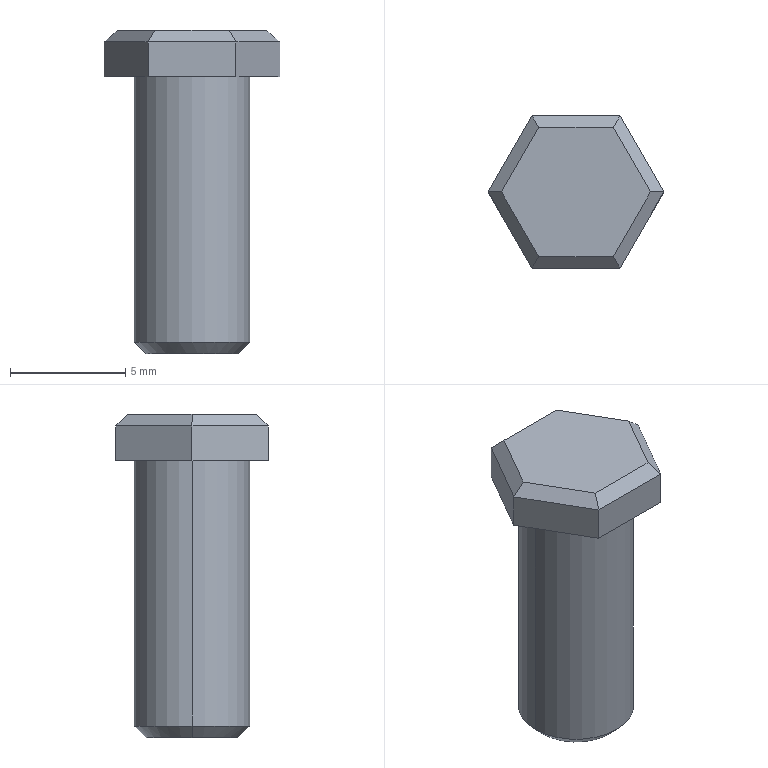Part | SolidWorks | features Chamfer 1, Extrusion 1, ICE 1 | 1 solid | 19 faces | box 7.616 x 6.595 x 14 mm | volume 306.418 mm3 | plane 15 | cone 2 | cylinder 2 | commonest cylinder face diameters 5 x2
STEP:
#1=CARTESIAN_POINT('',(718.,45.,-12.));
#2=VERTEX_POINT('',#1);
#3=CARTESIAN_POINT('',(722.,45.,-12.));
#4=VERTEX_POINT('',#3);
#5=CARTESIAN_POINT('',(720.,45.,-12.));
#6=DIRECTION('',(0.,0.,-1.));
#7=DIRECTION('',(1.,0.,0.));
#8=AXIS2_PLACEMENT_3D('',#5,#6,#7);
#9=CIRCLE('',#8,2.);
#10=EDGE_CURVE('',#2,#4,#9,.T.);
#11=ORIENTED_EDGE('',*,*,#10,.F.);
#12=CARTESIAN_POINT('',(717.5,45.,-11.5));
#13=VERTEX_POINT('',#12);
#14=CARTESIAN_POINT('',(717.5,45.,-11.5));
#15=DIRECTION('',(-0.7071,0.,0.7071));
#16=VECTOR('',#15,1000.);
#17=LINE('',#14,#16);
#18=EDGE_CURVE('',#2,#13,#17,.T.);
#19=ORIENTED_EDGE('',*,*,#18,.T.);
#20=CARTESIAN_POINT('',(722.5,45.,-11.5));
#21=VERTEX_POINT('',#20);
#22=CARTESIAN_POINT('',(720.,45.,-11.5));
#23=DIRECTION('',(0.,0.,1.));
#24=DIRECTION('',(1.,0.,0.));
#25=AXIS2_PLACEMENT_3D('',#22,#23,#24);
#26=CIRCLE('',#25,2.5);
#27=EDGE_CURVE('',#21,#13,#26,.T.);
#28=ORIENTED_EDGE('',*,*,#27,.F.);
#29=CARTESIAN_POINT('',(722.5,45.,-11.5));
#30=DIRECTION('',(0.7071,0.,0.7071));
#31=VECTOR('',#30,1000.);
#32=LINE('',#29,#31);
#33=EDGE_CURVE('',#4,#21,#32,.T.);
#34=ORIENTED_EDGE('',*,*,#33,.F.);
#35=EDGE_LOOP('',(#11,#19,#28,#34));
#36=FACE_OUTER_BOUND('',#35,.T.);
#37=CARTESIAN_POINT('',(720.,45.,-11.5));
#38=DIRECTION('',(0.,0.,1.));
#39=DIRECTION('',(1.,0.,0.));
#40=AXIS2_PLACEMENT_3D('',#37,#38,#39);
#41=CONICAL_SURFACE('',#40,2.5,0.7854);
#42=ADVANCED_FACE('',(#36),#41,.T.);
#43=ORIENTED_EDGE('',*,*,#27,.T.);
#44=CARTESIAN_POINT('',(717.5,45.,0.));
#45=VERTEX_POINT('',#44);
#46=CARTESIAN_POINT('',(717.5,45.,-12.));
#47=DIRECTION('',(0.,0.,1.));
#48=VECTOR('',#47,1000.);
#49=LINE('',#46,#48);
#50=EDGE_CURVE('',#13,#45,#49,.T.);
#51=ORIENTED_EDGE('',*,*,#50,.T.);
#52=CARTESIAN_POINT('',(722.5,45.,0.));
#53=VERTEX_POINT('',#52);
#54=CARTESIAN_POINT('',(720.,45.,0.));
#55=DIRECTION('',(0.,0.,1.));
#56=DIRECTION('',(1.,0.,0.));
#57=AXIS2_PLACEMENT_3D('',#54,#55,#56);
#58=CIRCLE('',#57,2.5);
#59=EDGE_CURVE('',#53,#45,#58,.T.);
#60=ORIENTED_EDGE('',*,*,#59,.F.);
#61=CARTESIAN_POINT('',(722.5,45.,-12.));
#62=DIRECTION('',(0.,0.,1.));
#63=VECTOR('',#62,1000.);
#64=LINE('',#61,#63);
#65=EDGE_CURVE('',#21,#53,#64,.T.);
#66=ORIENTED_EDGE('',*,*,#65,.F.);
#67=EDGE_LOOP('',(#43,#51,#60,#66));
#68=FACE_OUTER_BOUND('',#67,.T.);
#69=CARTESIAN_POINT('',(720.,45.,-12.));
#70=DIRECTION('',(0.,0.,1.));
#71=DIRECTION('',(1.,0.,0.));
#72=AXIS2_PLACEMENT_3D('',#69,#70,#71);
#73=CYLINDRICAL_SURFACE('',#72,2.5);
#74=ADVANCED_FACE('',(#68),#73,.T.);
#75=ORIENTED_EDGE('',*,*,#50,.F.);
#76=CARTESIAN_POINT('',(720.,45.,-11.5));
#77=DIRECTION('',(0.,0.,1.));
#78=DIRECTION('',(1.,0.,0.));
#79=AXIS2_PLACEMENT_3D('',#76,#77,#78);
#80=CIRCLE('',#79,2.5);
#81=EDGE_CURVE('',#13,#21,#80,.T.);
#82=ORIENTED_EDGE('',*,*,#81,.T.);
#83=ORIENTED_EDGE('',*,*,#65,.T.);
#84=CARTESIAN_POINT('',(720.,45.,0.));
#85=DIRECTION('',(0.,0.,1.));
#86=DIRECTION('',(1.,0.,0.));
#87=AXIS2_PLACEMENT_3D('',#84,#85,#86);
#88=CIRCLE('',#87,2.5);
#89=EDGE_CURVE('',#45,#53,#88,.T.);
#90=ORIENTED_EDGE('',*,*,#89,.F.);
#91=EDGE_LOOP('',(#75,#82,#83,#90));
#92=FACE_OUTER_BOUND('',#91,.T.);
#93=CARTESIAN_POINT('',(720.,45.,-12.));
#94=DIRECTION('',(0.,0.,1.));
#95=DIRECTION('',(1.,0.,0.));
#96=AXIS2_PLACEMENT_3D('',#93,#94,#95);
#97=CYLINDRICAL_SURFACE('',#96,2.5);
#98=ADVANCED_FACE('',(#92),#97,.T.);
#99=CARTESIAN_POINT('',(720.,45.,-12.));
#100=DIRECTION('',(0.,0.,-1.));
#101=DIRECTION('',(1.,0.,0.));
#102=AXIS2_PLACEMENT_3D('',#99,#100,#101);
#103=CIRCLE('',#102,2.);
#104=EDGE_CURVE('',#4,#2,#103,.T.);
#105=ORIENTED_EDGE('',*,*,#104,.T.);
#106=ORIENTED_EDGE('',*,*,#10,.T.);
#107=EDGE_LOOP('',(#105,#106));
#108=FACE_OUTER_BOUND('',#107,.T.);
#109=CARTESIAN_POINT('',(720.,45.,-12.));
#110=DIRECTION('',(0.,0.,1.));
#111=DIRECTION('',(1.,0.,0.));
#112=AXIS2_PLACEMENT_3D('',#109,#110,#111);
#113=PLANE('',#112);
#114=ADVANCED_FACE('',(#108),#113,.F.);
#115=CARTESIAN_POINT('',(718.096,41.702,1.5));
#116=VERTEX_POINT('',#115);
#117=CARTESIAN_POINT('',(718.096,41.702,0.));
#118=VERTEX_POINT('',#117);
#119=CARTESIAN_POINT('',(718.096,41.702,2.));
#120=DIRECTION('',(0.,0.,-1.));
#121=VECTOR('',#120,1000.);
#122=LINE('',#119,#121);
#123=EDGE_CURVE('',#116,#118,#122,.T.);
#124=ORIENTED_EDGE('',*,*,#123,.F.);
#125=CARTESIAN_POINT('',(716.192,45.,1.5));
#126=VERTEX_POINT('',#125);
#127=CARTESIAN_POINT('',(716.192,45.,1.5));
#128=DIRECTION('',(-0.5,0.866,0.));
#129=VECTOR('',#128,1000.);
#130=LINE('',#127,#129);
#131=EDGE_CURVE('',#116,#126,#130,.T.);
#132=ORIENTED_EDGE('',*,*,#131,.T.);
#133=CARTESIAN_POINT('',(716.192,45.,0.));
#134=VERTEX_POINT('',#133);
#135=CARTESIAN_POINT('',(716.192,45.,2.));
#136=DIRECTION('',(0.,0.,-1.));
#137=VECTOR('',#136,1000.);
#138=LINE('',#135,#137);
#139=EDGE_CURVE('',#126,#134,#138,.T.);
#140=ORIENTED_EDGE('',*,*,#139,.T.);
#141=CARTESIAN_POINT('',(716.192,45.,0.));
#142=DIRECTION('',(0.5,-0.866,0.));
#143=VECTOR('',#142,1000.);
#144=LINE('',#141,#143);
#145=EDGE_CURVE('',#134,#118,#144,.T.);
#146=ORIENTED_EDGE('',*,*,#145,.T.);
#147=EDGE_LOOP('',(#124,#132,#140,#146));
#148=FACE_OUTER_BOUND('',#147,.T.);
#149=CARTESIAN_POINT('',(716.192,45.,2.));
#150=DIRECTION('',(0.866,0.5,0.));
#151=DIRECTION('',(-0.5,0.866,0.));
#152=AXIS2_PLACEMENT_3D('',#149,#150,#151);
#153=PLANE('',#152);
#154=ADVANCED_FACE('',(#148),#153,.F.);
#155=CARTESIAN_POINT('',(721.904,41.702,1.5));
#156=VERTEX_POINT('',#155);
#157=CARTESIAN_POINT('',(721.904,41.702,0.));
#158=VERTEX_POINT('',#157);
#159=CARTESIAN_POINT('',(721.904,41.702,2.));
#160=DIRECTION('',(0.,0.,-1.));
#161=VECTOR('',#160,1000.);
#162=LINE('',#159,#161);
#163=EDGE_CURVE('',#156,#158,#162,.T.);
#164=ORIENTED_EDGE('',*,*,#163,.F.);
#165=CARTESIAN_POINT('',(718.096,41.702,1.5));
#166=DIRECTION('',(-1.,0.,0.));
#167=VECTOR('',#166,1000.);
#168=LINE('',#165,#167);
#169=EDGE_CURVE('',#156,#116,#168,.T.);
#170=ORIENTED_EDGE('',*,*,#169,.T.);
#171=ORIENTED_EDGE('',*,*,#123,.T.);
#172=CARTESIAN_POINT('',(718.096,41.702,0.));
#173=DIRECTION('',(1.,0.,0.));
#174=VECTOR('',#173,1000.);
#175=LINE('',#172,#174);
#176=EDGE_CURVE('',#118,#158,#175,.T.);
#177=ORIENTED_EDGE('',*,*,#176,.T.);
#178=EDGE_LOOP('',(#164,#170,#171,#177));
#179=FACE_OUTER_BOUND('',#178,.T.);
#180=CARTESIAN_POINT('',(718.096,41.702,2.));
#181=DIRECTION('',(0.,1.,0.));
#182=DIRECTION('',(-1.,0.,0.));
#183=AXIS2_PLACEMENT_3D('',#180,#181,#182);
#184=PLANE('',#183);
#185=ADVANCED_FACE('',(#179),#184,.F.);
#186=CARTESIAN_POINT('',(723.808,45.,1.5));
#187=VERTEX_POINT('',#186);
#188=CARTESIAN_POINT('',(723.808,45.,0.));
#189=VERTEX_POINT('',#188);
#190=CARTESIAN_POINT('',(723.808,45.,2.));
#191=DIRECTION('',(0.,0.,-1.));
#192=VECTOR('',#191,1000.);
#193=LINE('',#190,#192);
#194=EDGE_CURVE('',#187,#189,#193,.T.);
#195=ORIENTED_EDGE('',*,*,#194,.F.);
#196=CARTESIAN_POINT('',(721.904,41.702,1.5));
#197=DIRECTION('',(-0.5,-0.866,0.));
#198=VECTOR('',#197,1000.);
#199=LINE('',#196,#198);
#200=EDGE_CURVE('',#187,#156,#199,.T.);
#201=ORIENTED_EDGE('',*,*,#200,.T.);
#202=ORIENTED_EDGE('',*,*,#163,.T.);
#203=CARTESIAN_POINT('',(721.904,41.702,0.));
#204=DIRECTION('',(0.5,0.866,0.));
#205=VECTOR('',#204,1000.);
#206=LINE('',#203,#205);
#207=EDGE_CURVE('',#158,#189,#206,.T.);
#208=ORIENTED_EDGE('',*,*,#207,.T.);
#209=EDGE_LOOP('',(#195,#201,#202,#208));
#210=FACE_OUTER_BOUND('',#209,.T.);
#211=CARTESIAN_POINT('',(721.904,41.702,2.));
#212=DIRECTION('',(-0.866,0.5,0.));
#213=DIRECTION('',(-0.5,-0.866,0.));
#214=AXIS2_PLACEMENT_3D('',#211,#212,#213);
#215=PLANE('',#214);
#216=ADVANCED_FACE('',(#210),#215,.F.);
#217=CARTESIAN_POINT('',(721.904,48.298,1.5));
#218=VERTEX_POINT('',#217);
#219=CARTESIAN_POINT('',(721.904,48.298,0.));
#220=VERTEX_POINT('',#219);
#221=CARTESIAN_POINT('',(721.904,48.298,2.));
#222=DIRECTION('',(0.,0.,-1.));
#223=VECTOR('',#222,1000.);
#224=LINE('',#221,#223);
#225=EDGE_CURVE('',#218,#220,#224,.T.);
#226=ORIENTED_EDGE('',*,*,#225,.F.);
#227=CARTESIAN_POINT('',(723.808,45.,1.5));
#228=DIRECTION('',(0.5,-0.866,0.));
#229=VECTOR('',#228,1000.);
#230=LINE('',#227,#229);
#231=EDGE_CURVE('',#218,#187,#230,.T.);
#232=ORIENTED_EDGE('',*,*,#231,.T.);
#233=ORIENTED_EDGE('',*,*,#194,.T.);
#234=CARTESIAN_POINT('',(723.808,45.,0.));
#235=DIRECTION('',(-0.5,0.866,0.));
#236=VECTOR('',#235,1000.);
#237=LINE('',#234,#236);
#238=EDGE_CURVE('',#189,#220,#237,.T.);
#239=ORIENTED_EDGE('',*,*,#238,.T.);
#240=EDGE_LOOP('',(#226,#232,#233,#239));
#241=FACE_OUTER_BOUND('',#240,.T.);
#242=CARTESIAN_POINT('',(723.808,45.,2.));
#243=DIRECTION('',(-0.866,-0.5,0.));
#244=DIRECTION('',(0.5,-0.866,0.));
#245=AXIS2_PLACEMENT_3D('',#242,#243,#244);
#246=PLANE('',#245);
#247=ADVANCED_FACE('',(#241),#246,.F.);
#248=CARTESIAN_POINT('',(718.096,48.298,1.5));
#249=VERTEX_POINT('',#248);
#250=CARTESIAN_POINT('',(718.096,48.298,0.));
#251=VERTEX_POINT('',#250);
#252=CARTESIAN_POINT('',(718.096,48.298,2.));
#253=DIRECTION('',(0.,0.,-1.));
#254=VECTOR('',#253,1000.);
#255=LINE('',#252,#254);
#256=EDGE_CURVE('',#249,#251,#255,.T.);
#257=ORIENTED_EDGE('',*,*,#256,.F.);
#258=CARTESIAN_POINT('',(721.904,48.298,1.5));
#259=DIRECTION('',(1.,0.,0.));
#260=VECTOR('',#259,1000.);
#261=LINE('',#258,#260);
#262=EDGE_CURVE('',#249,#218,#261,.T.);
#263=ORIENTED_EDGE('',*,*,#262,.T.);
#264=ORIENTED_EDGE('',*,*,#225,.T.);
#265=CARTESIAN_POINT('',(721.904,48.298,0.));
#266=DIRECTION('',(-1.,0.,0.));
#267=VECTOR('',#266,1000.);
#268=LINE('',#265,#267);
#269=EDGE_CURVE('',#220,#251,#268,.T.);
#270=ORIENTED_EDGE('',*,*,#269,.T.);
#271=EDGE_LOOP('',(#257,#263,#264,#270));
#272=FACE_OUTER_BOUND('',#271,.T.);
#273=CARTESIAN_POINT('',(721.904,48.298,2.));
#274=DIRECTION('',(0.,-1.,0.));
#275=DIRECTION('',(1.,0.,0.));
#276=AXIS2_PLACEMENT_3D('',#273,#274,#275);
#277=PLANE('',#276);
#278=ADVANCED_FACE('',(#272),#277,.F.);
#279=ORIENTED_EDGE('',*,*,#139,.F.);
#280=CARTESIAN_POINT('',(718.096,48.298,1.5));
#281=DIRECTION('',(0.5,0.866,0.));
#282=VECTOR('',#281,1000.);
#283=LINE('',#280,#282);
#284=EDGE_CURVE('',#126,#249,#283,.T.);
#285=ORIENTED_EDGE('',*,*,#284,.T.);
#286=ORIENTED_EDGE('',*,*,#256,.T.);
#287=CARTESIAN_POINT('',(718.096,48.298,0.));
#288=DIRECTION('',(-0.5,-0.866,0.));
#289=VECTOR('',#288,1000.);
#290=LINE('',#287,#289);
#291=EDGE_CURVE('',#251,#134,#290,.T.);
#292=ORIENTED_EDGE('',*,*,#291,.T.);
#293=EDGE_LOOP('',(#279,#285,#286,#292));
#294=FACE_OUTER_BOUND('',#293,.T.);
#295=CARTESIAN_POINT('',(718.096,48.298,2.));
#296=DIRECTION('',(0.866,-0.5,0.));
#297=DIRECTION('',(0.5,0.866,0.));
#298=AXIS2_PLACEMENT_3D('',#295,#296,#297);
#299=PLANE('',#298);
#300=ADVANCED_FACE('',(#294),#299,.F.);
#301=CARTESIAN_POINT('',(721.615,47.798,2.));
#302=VERTEX_POINT('',#301);
#303=CARTESIAN_POINT('',(718.385,47.798,2.));
#304=VERTEX_POINT('',#303);
#305=CARTESIAN_POINT('',(718.096,47.798,2.));
#306=DIRECTION('',(-1.,0.,0.));
#307=VECTOR('',#306,1000.);
#308=LINE('',#305,#307);
#309=EDGE_CURVE('',#302,#304,#308,.T.);
#310=ORIENTED_EDGE('',*,*,#309,.T.);
#311=CARTESIAN_POINT('',(716.77,45.,2.));
#312=VERTEX_POINT('',#311);
#313=CARTESIAN_POINT('',(716.625,44.75,2.));
#314=DIRECTION('',(-0.5,-0.866,0.));
#315=VECTOR('',#314,1000.);
#316=LINE('',#313,#315);
#317=EDGE_CURVE('',#304,#312,#316,.T.);
#318=ORIENTED_EDGE('',*,*,#317,.T.);
#319=CARTESIAN_POINT('',(718.385,42.202,2.));
#320=VERTEX_POINT('',#319);
#321=CARTESIAN_POINT('',(718.529,41.952,2.));
#322=DIRECTION('',(0.5,-0.866,0.));
#323=VECTOR('',#322,1000.);
#324=LINE('',#321,#323);
#325=EDGE_CURVE('',#312,#320,#324,.T.);
#326=ORIENTED_EDGE('',*,*,#325,.T.);
#327=CARTESIAN_POINT('',(721.615,42.202,2.));
#328=VERTEX_POINT('',#327);
#329=CARTESIAN_POINT('',(721.904,42.202,2.));
#330=DIRECTION('',(1.,0.,0.));
#331=VECTOR('',#330,1000.);
#332=LINE('',#329,#331);
#333=EDGE_CURVE('',#320,#328,#332,.T.);
#334=ORIENTED_EDGE('',*,*,#333,.T.);
#335=CARTESIAN_POINT('',(723.23,45.,2.));
#336=VERTEX_POINT('',#335);
#337=CARTESIAN_POINT('',(723.375,45.25,2.));
#338=DIRECTION('',(0.5,0.866,0.));
#339=VECTOR('',#338,1000.);
#340=LINE('',#337,#339);
#341=EDGE_CURVE('',#328,#336,#340,.T.);
#342=ORIENTED_EDGE('',*,*,#341,.T.);
#343=CARTESIAN_POINT('',(721.471,48.048,2.));
#344=DIRECTION('',(-0.5,0.866,0.));
#345=VECTOR('',#344,1000.);
#346=LINE('',#343,#345);
#347=EDGE_CURVE('',#336,#302,#346,.T.);
#348=ORIENTED_EDGE('',*,*,#347,.T.);
#349=EDGE_LOOP('',(#310,#318,#326,#334,#342,#348));
#350=FACE_OUTER_BOUND('',#349,.T.);
#351=CARTESIAN_POINT('',(0.,0.,2.));
#352=DIRECTION('',(0.,0.,1.));
#353=DIRECTION('',(1.,0.,0.));
#354=AXIS2_PLACEMENT_3D('',#351,#352,#353);
#355=PLANE('',#354);
#356=ADVANCED_FACE('',(#350),#355,.T.);
#357=ORIENTED_EDGE('',*,*,#59,.T.);
#358=ORIENTED_EDGE('',*,*,#89,.T.);
#359=EDGE_LOOP('',(#357,#358));
#360=FACE_BOUND('',#359,.T.);
#361=ORIENTED_EDGE('',*,*,#145,.F.);
#362=ORIENTED_EDGE('',*,*,#291,.F.);
#363=ORIENTED_EDGE('',*,*,#269,.F.);
#364=ORIENTED_EDGE('',*,*,#238,.F.);
#365=ORIENTED_EDGE('',*,*,#207,.F.);
#366=ORIENTED_EDGE('',*,*,#176,.F.);
#367=EDGE_LOOP('',(#361,#362,#363,#364,#365,#366));
#368=FACE_OUTER_BOUND('',#367,.T.);
#369=CARTESIAN_POINT('',(0.,0.,0.));
#370=DIRECTION('',(0.,0.,1.));
#371=DIRECTION('',(1.,0.,0.));
#372=AXIS2_PLACEMENT_3D('',#369,#370,#371);
#373=PLANE('',#372);
#374=ADVANCED_FACE('',(#360,#368),#373,.F.);
#375=ORIENTED_EDGE('',*,*,#18,.F.);
#376=ORIENTED_EDGE('',*,*,#104,.F.);
#377=ORIENTED_EDGE('',*,*,#33,.T.);
#378=ORIENTED_EDGE('',*,*,#81,.F.);
#379=EDGE_LOOP('',(#375,#376,#377,#378));
#380=FACE_OUTER_BOUND('',#379,.T.);
#381=CARTESIAN_POINT('',(720.,45.,-11.5));
#382=DIRECTION('',(0.,0.,1.));
#383=DIRECTION('',(1.,0.,0.));
#384=AXIS2_PLACEMENT_3D('',#381,#382,#383);
#385=CONICAL_SURFACE('',#384,2.5,0.7854);
#386=ADVANCED_FACE('',(#380),#385,.T.);
#387=CARTESIAN_POINT('',(618.527,220.756,180.553));
#388=DIRECTION('',(-0.378,0.6547,0.6547));
#389=VECTOR('',#388,1000.);
#390=LINE('',#387,#389);
#391=EDGE_CURVE('',#156,#328,#390,.T.);
#392=ORIENTED_EDGE('',*,*,#391,.F.);
#393=ORIENTED_EDGE('',*,*,#200,.F.);
#394=CARTESIAN_POINT('',(608.777,45.,101.119));
#395=DIRECTION('',(0.7559,0.,-0.6547));
#396=VECTOR('',#395,1000.);
#397=LINE('',#394,#396);
#398=EDGE_CURVE('',#336,#187,#397,.T.);
#399=ORIENTED_EDGE('',*,*,#398,.F.);
#400=ORIENTED_EDGE('',*,*,#341,.F.);
#401=EDGE_LOOP('',(#392,#393,#399,#400));
#402=FACE_OUTER_BOUND('',#401,.T.);
#403=CARTESIAN_POINT('',(522.937,-301.918,2.));
#404=DIRECTION('',(0.6124,-0.3536,0.7071));
#405=DIRECTION('',(-0.5,-0.866,0.));
#406=AXIS2_PLACEMENT_3D('',#403,#404,#405);
#407=PLANE('',#406);
#408=ADVANCED_FACE('',(#402),#407,.T.);
#409=ORIENTED_EDGE('',*,*,#398,.T.);
#410=ORIENTED_EDGE('',*,*,#231,.F.);
#411=CARTESIAN_POINT('',(767.246,126.832,-77.034));
#412=DIRECTION('',(0.378,0.6547,-0.6547));
#413=VECTOR('',#412,1000.);
#414=LINE('',#411,#413);
#415=EDGE_CURVE('',#302,#218,#414,.T.);
#416=ORIENTED_EDGE('',*,*,#415,.F.);
#417=ORIENTED_EDGE('',*,*,#347,.F.);
#418=EDGE_LOOP('',(#409,#410,#416,#417));
#419=FACE_OUTER_BOUND('',#418,.T.);
#420=CARTESIAN_POINT('',(561.908,324.418,2.));
#421=DIRECTION('',(0.6124,0.3536,0.7071));
#422=DIRECTION('',(0.5,-0.866,0.));
#423=AXIS2_PLACEMENT_3D('',#420,#421,#422);
#424=PLANE('',#423);
#425=ADVANCED_FACE('',(#419),#424,.T.);
#426=ORIENTED_EDGE('',*,*,#391,.T.);
#427=ORIENTED_EDGE('',*,*,#333,.F.);
#428=CARTESIAN_POINT('',(764.477,122.036,81.834));
#429=DIRECTION('',(0.378,0.6547,0.6547));
#430=VECTOR('',#429,1000.);
#431=LINE('',#428,#430);
#432=EDGE_CURVE('',#116,#320,#431,.T.);
#433=ORIENTED_EDGE('',*,*,#432,.F.);
#434=ORIENTED_EDGE('',*,*,#169,.F.);
#435=EDGE_LOOP('',(#426,#427,#433,#434));
#436=FACE_OUTER_BOUND('',#435,.T.);
#437=CARTESIAN_POINT('',(0.,42.202,2.));
#438=DIRECTION('',(0.,-0.7071,0.7071));
#439=DIRECTION('',(-1.,0.,0.));
#440=AXIS2_PLACEMENT_3D('',#437,#438,#439);
#441=PLANE('',#440);
#442=ADVANCED_FACE('',(#436),#441,.T.);
#443=ORIENTED_EDGE('',*,*,#415,.T.);
#444=ORIENTED_EDGE('',*,*,#262,.F.);
#445=CARTESIAN_POINT('',(615.758,225.552,-175.754));
#446=DIRECTION('',(-0.378,0.6547,-0.6547));
#447=VECTOR('',#446,1000.);
#448=LINE('',#445,#447);
#449=EDGE_CURVE('',#304,#249,#448,.T.);
#450=ORIENTED_EDGE('',*,*,#449,.F.);
#451=ORIENTED_EDGE('',*,*,#309,.F.);
#452=EDGE_LOOP('',(#443,#444,#450,#451));
#453=FACE_OUTER_BOUND('',#452,.T.);
#454=CARTESIAN_POINT('',(0.,47.798,2.));
#455=DIRECTION('',(0.,0.7071,0.7071));
#456=DIRECTION('',(1.,0.,0.));
#457=AXIS2_PLACEMENT_3D('',#454,#455,#456);
#458=PLANE('',#457);
#459=ADVANCED_FACE('',(#453),#458,.T.);
#460=ORIENTED_EDGE('',*,*,#432,.T.);
#461=ORIENTED_EDGE('',*,*,#325,.F.);
#462=CARTESIAN_POINT('',(625.508,45.,-77.034));
#463=DIRECTION('',(0.7559,0.,0.6547));
#464=VECTOR('',#463,1000.);
#465=LINE('',#462,#464);
#466=EDGE_CURVE('',#126,#312,#465,.T.);
#467=ORIENTED_EDGE('',*,*,#466,.F.);
#468=ORIENTED_EDGE('',*,*,#131,.F.);
#469=EDGE_LOOP('',(#460,#461,#467,#468));
#470=FACE_OUTER_BOUND('',#469,.T.);
#471=CARTESIAN_POINT('',(557.063,321.62,2.));
#472=DIRECTION('',(-0.6124,-0.3536,0.7071));
#473=DIRECTION('',(-0.5,0.866,0.));
#474=AXIS2_PLACEMENT_3D('',#471,#472,#473);
#475=PLANE('',#474);
#476=ADVANCED_FACE('',(#470),#475,.T.);
#477=ORIENTED_EDGE('',*,*,#449,.T.);
#478=ORIENTED_EDGE('',*,*,#284,.F.);
#479=ORIENTED_EDGE('',*,*,#466,.T.);
#480=ORIENTED_EDGE('',*,*,#317,.F.);
#481=EDGE_LOOP('',(#477,#478,#479,#480));
#482=FACE_OUTER_BOUND('',#481,.T.);
#483=CARTESIAN_POINT('',(518.092,-299.12,2.));
#484=DIRECTION('',(-0.6124,0.3536,0.7071));
#485=DIRECTION('',(0.5,0.866,0.));
#486=AXIS2_PLACEMENT_3D('',#483,#484,#485);
#487=PLANE('',#486);
#488=ADVANCED_FACE('',(#482),#487,.T.);
#489=CLOSED_SHELL('',(#42,#74,#98,#114,#154,#185,#216,#247,#278,#300,#356,#374,#386,#408,#425,#442,#459,#476,#488));
#490=MANIFOLD_SOLID_BREP('',#489);
#491=CARTESIAN_POINT('',(0.,0.,0.));
#492=DIRECTION('',(0.,0.,1.));
#493=DIRECTION('',(1.,0.,0.));
#494=AXIS2_PLACEMENT_3D('',#491,#492,#493);
#495=(LENGTH_UNIT()NAMED_UNIT(*)SI_UNIT(.MILLI.,.METRE.));
#496=UNCERTAINTY_MEASURE_WITH_UNIT(LENGTH_MEASURE(0.00001),#495,'','');
#497=(NAMED_UNIT(*)PLANE_ANGLE_UNIT()SI_UNIT($,.RADIAN.));
#498=(NAMED_UNIT(*)SI_UNIT($,.STERADIAN.)SOLID_ANGLE_UNIT());
#499=(GEOMETRIC_REPRESENTATION_CONTEXT(3)GLOBAL_UNCERTAINTY_ASSIGNED_CONTEXT((#496))GLOBAL_UNIT_ASSIGNED_CONTEXT((#495,#497,#498))REPRESENTATION_CONTEXT('',''));
#500=ADVANCED_BREP_SHAPE_REPRESENTATION('',(#490,#494),#499);